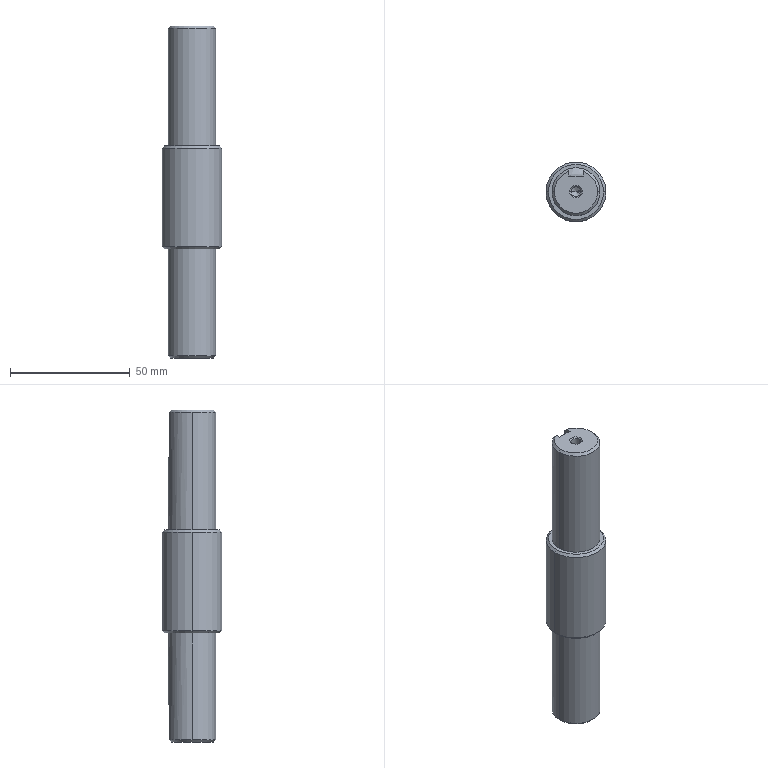Part | SolidWorks | features BaseBody 1 | 1 solid | 40 faces | box 25 x 25 x 138.5 mm | volume 49958 mm3 | cone 18 | cylinder 10 | plane 10 | spline 2 | commonest cylinder face diameters 4.2 x4 20 x4 25 x2
STEP:
#1=CARTESIAN_POINT('',(2.1,0.,-66.5));
#2=VERTEX_POINT('',#1);
#3=CARTESIAN_POINT('',(-2.1,0.,-66.5));
#4=VERTEX_POINT('',#3);
#5=CARTESIAN_POINT('',(0.,0.,-66.5));
#6=DIRECTION('',(0.,0.,-1.));
#7=DIRECTION('',(-1.,0.,0.));
#8=AXIS2_PLACEMENT_3D('',#5,#6,#7);
#9=CIRCLE('',#8,2.1);
#10=EDGE_CURVE('',#2,#4,#9,.T.);
#11=ORIENTED_EDGE('',*,*,#10,.F.);
#12=CARTESIAN_POINT('',(2.6,0.,-67.));
#13=VERTEX_POINT('',#12);
#14=CARTESIAN_POINT('',(2.1,0.,-66.5));
#15=DIRECTION('',(0.7071,0.,-0.7071));
#16=VECTOR('',#15,1000.);
#17=LINE('',#14,#16);
#18=EDGE_CURVE('',#2,#13,#17,.T.);
#19=ORIENTED_EDGE('',*,*,#18,.T.);
#20=CARTESIAN_POINT('',(-2.6,0.,-67.));
#21=VERTEX_POINT('',#20);
#22=CARTESIAN_POINT('',(0.,0.,-67.));
#23=DIRECTION('',(0.,0.,1.));
#24=DIRECTION('',(-1.,0.,0.));
#25=AXIS2_PLACEMENT_3D('',#22,#23,#24);
#26=CIRCLE('',#25,2.6);
#27=EDGE_CURVE('',#21,#13,#26,.T.);
#28=ORIENTED_EDGE('',*,*,#27,.F.);
#29=CARTESIAN_POINT('',(-2.1,0.,-66.5));
#30=DIRECTION('',(-0.7071,0.,-0.7071));
#31=VECTOR('',#30,1000.);
#32=LINE('',#29,#31);
#33=EDGE_CURVE('',#4,#21,#32,.T.);
#34=ORIENTED_EDGE('',*,*,#33,.F.);
#35=EDGE_LOOP('',(#11,#19,#28,#34));
#36=FACE_OUTER_BOUND('',#35,.T.);
#37=CARTESIAN_POINT('',(0.,0.,-66.5));
#38=DIRECTION('',(0.,0.,-1.));
#39=DIRECTION('',(-1.,0.,0.));
#40=AXIS2_PLACEMENT_3D('',#37,#38,#39);
#41=CONICAL_SURFACE('',#40,2.1,0.7854);
#42=ADVANCED_FACE('',(#36),#41,.F.);
#43=CARTESIAN_POINT('',(-2.1,0.,71.));
#44=VERTEX_POINT('',#43);
#45=CARTESIAN_POINT('',(2.1,0.,71.));
#46=VERTEX_POINT('',#45);
#47=CARTESIAN_POINT('',(0.,0.,71.));
#48=DIRECTION('',(0.,0.,1.));
#49=DIRECTION('',(1.,0.,0.));
#50=AXIS2_PLACEMENT_3D('',#47,#48,#49);
#51=CIRCLE('',#50,2.1);
#52=EDGE_CURVE('',#44,#46,#51,.T.);
#53=ORIENTED_EDGE('',*,*,#52,.F.);
#54=CARTESIAN_POINT('',(-2.6,0.,71.5));
#55=VERTEX_POINT('',#54);
#56=CARTESIAN_POINT('',(-2.1,0.,71.));
#57=DIRECTION('',(-0.7071,0.,0.7071));
#58=VECTOR('',#57,1000.);
#59=LINE('',#56,#58);
#60=EDGE_CURVE('',#44,#55,#59,.T.);
#61=ORIENTED_EDGE('',*,*,#60,.T.);
#62=CARTESIAN_POINT('',(2.6,0.,71.5));
#63=VERTEX_POINT('',#62);
#64=CARTESIAN_POINT('',(0.,0.,71.5));
#65=DIRECTION('',(0.,0.,-1.));
#66=DIRECTION('',(1.,0.,0.));
#67=AXIS2_PLACEMENT_3D('',#64,#65,#66);
#68=CIRCLE('',#67,2.6);
#69=EDGE_CURVE('',#63,#55,#68,.T.);
#70=ORIENTED_EDGE('',*,*,#69,.F.);
#71=CARTESIAN_POINT('',(2.1,0.,71.));
#72=DIRECTION('',(0.7071,0.,0.7071));
#73=VECTOR('',#72,1000.);
#74=LINE('',#71,#73);
#75=EDGE_CURVE('',#46,#63,#74,.T.);
#76=ORIENTED_EDGE('',*,*,#75,.F.);
#77=EDGE_LOOP('',(#53,#61,#70,#76));
#78=FACE_OUTER_BOUND('',#77,.T.);
#79=CARTESIAN_POINT('',(0.,0.,71.));
#80=DIRECTION('',(0.,0.,1.));
#81=DIRECTION('',(1.,0.,0.));
#82=AXIS2_PLACEMENT_3D('',#79,#80,#81);
#83=CONICAL_SURFACE('',#82,2.1,0.7854);
#84=ADVANCED_FACE('',(#78),#83,.F.);
#85=CARTESIAN_POINT('',(-2.1,0.,59.1));
#86=VERTEX_POINT('',#85);
#87=CARTESIAN_POINT('',(2.1,0.,59.1));
#88=VERTEX_POINT('',#87);
#89=CARTESIAN_POINT('',(0.,0.,59.1));
#90=DIRECTION('',(0.,0.,1.));
#91=DIRECTION('',(1.,0.,0.));
#92=AXIS2_PLACEMENT_3D('',#89,#90,#91);
#93=CIRCLE('',#92,2.1);
#94=EDGE_CURVE('',#86,#88,#93,.T.);
#95=ORIENTED_EDGE('',*,*,#94,.F.);
#96=CARTESIAN_POINT('',(-2.1,0.,71.5));
#97=DIRECTION('',(0.,0.,1.));
#98=VECTOR('',#97,1000.);
#99=LINE('',#96,#98);
#100=EDGE_CURVE('',#86,#44,#99,.T.);
#101=ORIENTED_EDGE('',*,*,#100,.T.);
#102=ORIENTED_EDGE('',*,*,#52,.T.);
#103=CARTESIAN_POINT('',(2.1,0.,71.5));
#104=DIRECTION('',(0.,0.,1.));
#105=VECTOR('',#104,1000.);
#106=LINE('',#103,#105);
#107=EDGE_CURVE('',#88,#46,#106,.T.);
#108=ORIENTED_EDGE('',*,*,#107,.F.);
#109=EDGE_LOOP('',(#95,#101,#102,#108));
#110=FACE_OUTER_BOUND('',#109,.T.);
#111=CARTESIAN_POINT('',(0.,0.,71.5));
#112=DIRECTION('',(0.,0.,1.));
#113=DIRECTION('',(1.,0.,0.));
#114=AXIS2_PLACEMENT_3D('',#111,#112,#113);
#115=CYLINDRICAL_SURFACE('',#114,2.1);
#116=ADVANCED_FACE('',(#110),#115,.F.);
#117=CARTESIAN_POINT('',(0.,0.,57.838));
#118=VERTEX_POINT('',#117);
#119=CARTESIAN_POINT('',(2.1,0.,59.1));
#120=DIRECTION('',(0.8572,0.,0.515));
#121=VECTOR('',#120,1000.);
#122=LINE('',#119,#121);
#123=EDGE_CURVE('',#118,#88,#122,.T.);
#124=ORIENTED_EDGE('',*,*,#123,.F.);
#125=CARTESIAN_POINT('',(-2.1,0.,59.1));
#126=DIRECTION('',(-0.8572,0.,0.515));
#127=VECTOR('',#126,1000.);
#128=LINE('',#125,#127);
#129=EDGE_CURVE('',#118,#86,#128,.T.);
#130=ORIENTED_EDGE('',*,*,#129,.T.);
#131=ORIENTED_EDGE('',*,*,#94,.T.);
#132=EDGE_LOOP('',(#124,#130,#131));
#133=FACE_OUTER_BOUND('',#132,.T.);
#134=CARTESIAN_POINT('',(0.,0.,59.1));
#135=DIRECTION('',(0.,0.,1.));
#136=DIRECTION('',(1.,0.,0.));
#137=AXIS2_PLACEMENT_3D('',#134,#135,#136);
#138=CONICAL_SURFACE('',#137,2.1,1.03);
#139=ADVANCED_FACE('',(#133),#138,.F.);
#140=CARTESIAN_POINT('',(2.1,0.,-54.6));
#141=VERTEX_POINT('',#140);
#142=CARTESIAN_POINT('',(-2.1,0.,-54.6));
#143=VERTEX_POINT('',#142);
#144=CARTESIAN_POINT('',(0.,0.,-54.6));
#145=DIRECTION('',(0.,0.,-1.));
#146=DIRECTION('',(-1.,0.,0.));
#147=AXIS2_PLACEMENT_3D('',#144,#145,#146);
#148=CIRCLE('',#147,2.1);
#149=EDGE_CURVE('',#141,#143,#148,.T.);
#150=ORIENTED_EDGE('',*,*,#149,.F.);
#151=CARTESIAN_POINT('',(2.1,0.,-67.));
#152=DIRECTION('',(0.,0.,-1.));
#153=VECTOR('',#152,1000.);
#154=LINE('',#151,#153);
#155=EDGE_CURVE('',#141,#2,#154,.T.);
#156=ORIENTED_EDGE('',*,*,#155,.T.);
#157=ORIENTED_EDGE('',*,*,#10,.T.);
#158=CARTESIAN_POINT('',(-2.1,0.,-67.));
#159=DIRECTION('',(0.,0.,-1.));
#160=VECTOR('',#159,1000.);
#161=LINE('',#158,#160);
#162=EDGE_CURVE('',#143,#4,#161,.T.);
#163=ORIENTED_EDGE('',*,*,#162,.F.);
#164=EDGE_LOOP('',(#150,#156,#157,#163));
#165=FACE_OUTER_BOUND('',#164,.T.);
#166=CARTESIAN_POINT('',(0.,0.,-67.));
#167=DIRECTION('',(0.,0.,-1.));
#168=DIRECTION('',(-1.,0.,0.));
#169=AXIS2_PLACEMENT_3D('',#166,#167,#168);
#170=CYLINDRICAL_SURFACE('',#169,2.1);
#171=ADVANCED_FACE('',(#165),#170,.F.);
#172=CARTESIAN_POINT('',(0.,0.,-53.338));
#173=VERTEX_POINT('',#172);
#174=CARTESIAN_POINT('',(-2.1,0.,-54.6));
#175=DIRECTION('',(-0.8572,0.,-0.515));
#176=VECTOR('',#175,1000.);
#177=LINE('',#174,#176);
#178=EDGE_CURVE('',#173,#143,#177,.T.);
#179=ORIENTED_EDGE('',*,*,#178,.F.);
#180=CARTESIAN_POINT('',(2.1,0.,-54.6));
#181=DIRECTION('',(0.8572,0.,-0.515));
#182=VECTOR('',#181,1000.);
#183=LINE('',#180,#182);
#184=EDGE_CURVE('',#173,#141,#183,.T.);
#185=ORIENTED_EDGE('',*,*,#184,.T.);
#186=ORIENTED_EDGE('',*,*,#149,.T.);
#187=EDGE_LOOP('',(#179,#185,#186));
#188=FACE_OUTER_BOUND('',#187,.T.);
#189=CARTESIAN_POINT('',(0.,0.,-54.6));
#190=DIRECTION('',(0.,0.,-1.));
#191=DIRECTION('',(-1.,0.,0.));
#192=AXIS2_PLACEMENT_3D('',#189,#190,#191);
#193=CONICAL_SURFACE('',#192,2.1,1.03);
#194=ADVANCED_FACE('',(#188),#193,.F.);
#195=CARTESIAN_POINT('',(-9.,0.,-67.));
#196=VERTEX_POINT('',#195);
#197=CARTESIAN_POINT('',(-3.,8.485,-67.));
#198=VERTEX_POINT('',#197);
#199=CARTESIAN_POINT('',(0.,0.,-67.));
#200=DIRECTION('',(0.,0.,-1.));
#201=DIRECTION('',(-1.,0.,0.));
#202=AXIS2_PLACEMENT_3D('',#199,#200,#201);
#203=CIRCLE('',#202,9.);
#204=EDGE_CURVE('',#196,#198,#203,.T.);
#205=ORIENTED_EDGE('',*,*,#204,.F.);
#206=CARTESIAN_POINT('',(-10.,0.,-66.));
#207=VERTEX_POINT('',#206);
#208=CARTESIAN_POINT('',(-10.,0.,-66.));
#209=DIRECTION('',(-0.7071,0.,0.7071));
#210=VECTOR('',#209,1000.);
#211=LINE('',#208,#210);
#212=EDGE_CURVE('',#196,#207,#211,.T.);
#213=ORIENTED_EDGE('',*,*,#212,.T.);
#214=CARTESIAN_POINT('',(-3.,9.539,-66.));
#215=VERTEX_POINT('',#214);
#216=CARTESIAN_POINT('',(0.,0.,-66.));
#217=DIRECTION('',(0.,0.,1.));
#218=DIRECTION('',(-1.,0.,0.));
#219=AXIS2_PLACEMENT_3D('',#216,#217,#218);
#220=CIRCLE('',#219,10.);
#221=EDGE_CURVE('',#215,#207,#220,.T.);
#222=ORIENTED_EDGE('',*,*,#221,.F.);
#223=CARTESIAN_POINT('',(-3.,8.485,-67.));
#224=CARTESIAN_POINT('',(-3.,8.838,-66.668));
#225=CARTESIAN_POINT('',(-3.,9.189,-66.334));
#226=CARTESIAN_POINT('',(-3.,9.539,-66.));
#227=B_SPLINE_CURVE_WITH_KNOTS('',3,(#223,#224,#225,#226),.UNSPECIFIED.,.F.,.F.,(4,4),(0.,0.001453),.UNSPECIFIED.);
#228=EDGE_CURVE('',#198,#215,#227,.T.);
#229=ORIENTED_EDGE('',*,*,#228,.F.);
#230=EDGE_LOOP('',(#205,#213,#222,#229));
#231=FACE_OUTER_BOUND('',#230,.T.);
#232=CARTESIAN_POINT('',(0.,0.,-66.));
#233=DIRECTION('',(0.,0.,1.));
#234=DIRECTION('',(1.,0.,0.));
#235=AXIS2_PLACEMENT_3D('',#232,#233,#234);
#236=CONICAL_SURFACE('',#235,10.,0.7854);
#237=ADVANCED_FACE('',(#231),#236,.T.);
#238=ORIENTED_EDGE('',*,*,#212,.F.);
#239=CARTESIAN_POINT('',(9.,0.,-67.));
#240=VERTEX_POINT('',#239);
#241=CARTESIAN_POINT('',(0.,0.,-67.));
#242=DIRECTION('',(0.,0.,-1.));
#243=DIRECTION('',(-1.,0.,0.));
#244=AXIS2_PLACEMENT_3D('',#241,#242,#243);
#245=CIRCLE('',#244,9.);
#246=EDGE_CURVE('',#240,#196,#245,.T.);
#247=ORIENTED_EDGE('',*,*,#246,.F.);
#248=CARTESIAN_POINT('',(10.,0.,-66.));
#249=VERTEX_POINT('',#248);
#250=CARTESIAN_POINT('',(10.,0.,-66.));
#251=DIRECTION('',(0.7071,0.,0.7071));
#252=VECTOR('',#251,1000.);
#253=LINE('',#250,#252);
#254=EDGE_CURVE('',#240,#249,#253,.T.);
#255=ORIENTED_EDGE('',*,*,#254,.T.);
#256=CARTESIAN_POINT('',(0.,0.,-66.));
#257=DIRECTION('',(0.,0.,1.));
#258=DIRECTION('',(-1.,0.,0.));
#259=AXIS2_PLACEMENT_3D('',#256,#257,#258);
#260=CIRCLE('',#259,10.);
#261=EDGE_CURVE('',#207,#249,#260,.T.);
#262=ORIENTED_EDGE('',*,*,#261,.F.);
#263=EDGE_LOOP('',(#238,#247,#255,#262));
#264=FACE_OUTER_BOUND('',#263,.T.);
#265=CARTESIAN_POINT('',(0.,0.,-66.));
#266=DIRECTION('',(0.,0.,1.));
#267=DIRECTION('',(1.,0.,0.));
#268=AXIS2_PLACEMENT_3D('',#265,#266,#267);
#269=CONICAL_SURFACE('',#268,10.,0.7854);
#270=ADVANCED_FACE('',(#264),#269,.T.);
#271=CARTESIAN_POINT('',(11.5,0.,21.5));
#272=VERTEX_POINT('',#271);
#273=CARTESIAN_POINT('',(-11.5,0.,21.5));
#274=VERTEX_POINT('',#273);
#275=CARTESIAN_POINT('',(0.,0.,21.5));
#276=DIRECTION('',(0.,0.,1.));
#277=DIRECTION('',(1.,0.,0.));
#278=AXIS2_PLACEMENT_3D('',#275,#276,#277);
#279=CIRCLE('',#278,11.5);
#280=EDGE_CURVE('',#272,#274,#279,.T.);
#281=ORIENTED_EDGE('',*,*,#280,.F.);
#282=CARTESIAN_POINT('',(12.5,0.,20.5));
#283=VERTEX_POINT('',#282);
#284=CARTESIAN_POINT('',(11.5,0.,21.5));
#285=DIRECTION('',(0.7071,0.,-0.7071));
#286=VECTOR('',#285,1000.);
#287=LINE('',#284,#286);
#288=EDGE_CURVE('',#272,#283,#287,.T.);
#289=ORIENTED_EDGE('',*,*,#288,.T.);
#290=CARTESIAN_POINT('',(-12.5,0.,20.5));
#291=VERTEX_POINT('',#290);
#292=CARTESIAN_POINT('',(0.,0.,20.5));
#293=DIRECTION('',(0.,0.,-1.));
#294=DIRECTION('',(1.,0.,0.));
#295=AXIS2_PLACEMENT_3D('',#292,#293,#294);
#296=CIRCLE('',#295,12.5);
#297=EDGE_CURVE('',#291,#283,#296,.T.);
#298=ORIENTED_EDGE('',*,*,#297,.F.);
#299=CARTESIAN_POINT('',(-11.5,0.,21.5));
#300=DIRECTION('',(-0.7071,0.,-0.7071));
#301=VECTOR('',#300,1000.);
#302=LINE('',#299,#301);
#303=EDGE_CURVE('',#274,#291,#302,.T.);
#304=ORIENTED_EDGE('',*,*,#303,.F.);
#305=EDGE_LOOP('',(#281,#289,#298,#304));
#306=FACE_OUTER_BOUND('',#305,.T.);
#307=CARTESIAN_POINT('',(0.,0.,21.5));
#308=DIRECTION('',(0.,0.,-1.));
#309=DIRECTION('',(-1.,0.,0.));
#310=AXIS2_PLACEMENT_3D('',#307,#308,#309);
#311=CONICAL_SURFACE('',#310,11.5,0.7854);
#312=ADVANCED_FACE('',(#306),#311,.T.);
#313=CARTESIAN_POINT('',(-11.5,0.,-21.5));
#314=VERTEX_POINT('',#313);
#315=CARTESIAN_POINT('',(11.5,0.,-21.5));
#316=VERTEX_POINT('',#315);
#317=CARTESIAN_POINT('',(0.,0.,-21.5));
#318=DIRECTION('',(0.,0.,-1.));
#319=DIRECTION('',(1.,0.,0.));
#320=AXIS2_PLACEMENT_3D('',#317,#318,#319);
#321=CIRCLE('',#320,11.5);
#322=EDGE_CURVE('',#314,#316,#321,.T.);
#323=ORIENTED_EDGE('',*,*,#322,.F.);
#324=CARTESIAN_POINT('',(-12.5,0.,-20.5));
#325=VERTEX_POINT('',#324);
#326=CARTESIAN_POINT('',(-12.5,0.,-20.5));
#327=DIRECTION('',(-0.7071,0.,0.7071));
#328=VECTOR('',#327,1000.);
#329=LINE('',#326,#328);
#330=EDGE_CURVE('',#314,#325,#329,.T.);
#331=ORIENTED_EDGE('',*,*,#330,.T.);
#332=CARTESIAN_POINT('',(12.5,0.,-20.5));
#333=VERTEX_POINT('',#332);
#334=CARTESIAN_POINT('',(0.,0.,-20.5));
#335=DIRECTION('',(0.,0.,1.));
#336=DIRECTION('',(1.,0.,0.));
#337=AXIS2_PLACEMENT_3D('',#334,#335,#336);
#338=CIRCLE('',#337,12.5);
#339=EDGE_CURVE('',#333,#325,#338,.T.);
#340=ORIENTED_EDGE('',*,*,#339,.F.);
#341=CARTESIAN_POINT('',(12.5,0.,-20.5));
#342=DIRECTION('',(0.7071,0.,0.7071));
#343=VECTOR('',#342,1000.);
#344=LINE('',#341,#343);
#345=EDGE_CURVE('',#316,#333,#344,.T.);
#346=ORIENTED_EDGE('',*,*,#345,.F.);
#347=EDGE_LOOP('',(#323,#331,#340,#346));
#348=FACE_OUTER_BOUND('',#347,.T.);
#349=CARTESIAN_POINT('',(0.,0.,-20.5));
#350=DIRECTION('',(0.,0.,1.));
#351=DIRECTION('',(1.,0.,0.));
#352=AXIS2_PLACEMENT_3D('',#349,#350,#351);
#353=CONICAL_SURFACE('',#352,12.5,0.7854);
#354=ADVANCED_FACE('',(#348),#353,.T.);
#355=CARTESIAN_POINT('',(9.,0.,71.5));
#356=VERTEX_POINT('',#355);
#357=CARTESIAN_POINT('',(3.,8.485,71.5));
#358=VERTEX_POINT('',#357);
#359=CARTESIAN_POINT('',(0.,0.,71.5));
#360=DIRECTION('',(0.,0.,1.));
#361=DIRECTION('',(1.,0.,0.));
#362=AXIS2_PLACEMENT_3D('',#359,#360,#361);
#363=CIRCLE('',#362,9.);
#364=EDGE_CURVE('',#356,#358,#363,.T.);
#365=ORIENTED_EDGE('',*,*,#364,.F.);
#366=CARTESIAN_POINT('',(10.,0.,70.5));
#367=VERTEX_POINT('',#366);
#368=CARTESIAN_POINT('',(9.,0.,71.5));
#369=DIRECTION('',(0.7071,0.,-0.7071));
#370=VECTOR('',#369,1000.);
#371=LINE('',#368,#370);
#372=EDGE_CURVE('',#356,#367,#371,.T.);
#373=ORIENTED_EDGE('',*,*,#372,.T.);
#374=CARTESIAN_POINT('',(3.,9.539,70.5));
#375=VERTEX_POINT('',#374);
#376=CARTESIAN_POINT('',(0.,0.,70.5));
#377=DIRECTION('',(0.,0.,-1.));
#378=DIRECTION('',(1.,0.,0.));
#379=AXIS2_PLACEMENT_3D('',#376,#377,#378);
#380=CIRCLE('',#379,10.);
#381=EDGE_CURVE('',#375,#367,#380,.T.);
#382=ORIENTED_EDGE('',*,*,#381,.F.);
#383=CARTESIAN_POINT('',(3.,8.485,71.5));
#384=CARTESIAN_POINT('',(3.,8.838,71.168));
#385=CARTESIAN_POINT('',(3.,9.189,70.834));
#386=CARTESIAN_POINT('',(3.,9.539,70.5));
#387=B_SPLINE_CURVE_WITH_KNOTS('',3,(#383,#384,#385,#386),.UNSPECIFIED.,.F.,.F.,(4,4),(0.006491,0.007944),.UNSPECIFIED.);
#388=EDGE_CURVE('',#358,#375,#387,.T.);
#389=ORIENTED_EDGE('',*,*,#388,.F.);
#390=EDGE_LOOP('',(#365,#373,#382,#389));
#391=FACE_OUTER_BOUND('',#390,.T.);
#392=CARTESIAN_POINT('',(0.,0.,71.5));
#393=DIRECTION('',(0.,0.,-1.));
#394=DIRECTION('',(-1.,0.,0.));
#395=AXIS2_PLACEMENT_3D('',#392,#393,#394);
#396=CONICAL_SURFACE('',#395,9.,0.7854);
#397=ADVANCED_FACE('',(#391),#396,.T.);
#398=ORIENTED_EDGE('',*,*,#372,.F.);
#399=CARTESIAN_POINT('',(-9.,0.,71.5));
#400=VERTEX_POINT('',#399);
#401=CARTESIAN_POINT('',(0.,0.,71.5));
#402=DIRECTION('',(0.,0.,1.));
#403=DIRECTION('',(1.,0.,0.));
#404=AXIS2_PLACEMENT_3D('',#401,#402,#403);
#405=CIRCLE('',#404,9.);
#406=EDGE_CURVE('',#400,#356,#405,.T.);
#407=ORIENTED_EDGE('',*,*,#406,.F.);
#408=CARTESIAN_POINT('',(-10.,0.,70.5));
#409=VERTEX_POINT('',#408);
#410=CARTESIAN_POINT('',(-9.,0.,71.5));
#411=DIRECTION('',(-0.7071,0.,-0.7071));
#412=VECTOR('',#411,1000.);
#413=LINE('',#410,#412);
#414=EDGE_CURVE('',#400,#409,#413,.T.);
#415=ORIENTED_EDGE('',*,*,#414,.T.);
#416=CARTESIAN_POINT('',(0.,0.,70.5));
#417=DIRECTION('',(0.,0.,-1.));
#418=DIRECTION('',(1.,0.,0.));
#419=AXIS2_PLACEMENT_3D('',#416,#417,#418);
#420=CIRCLE('',#419,10.);
#421=EDGE_CURVE('',#367,#409,#420,.T.);
#422=ORIENTED_EDGE('',*,*,#421,.F.);
#423=EDGE_LOOP('',(#398,#407,#415,#422));
#424=FACE_OUTER_BOUND('',#423,.T.);
#425=CARTESIAN_POINT('',(0.,0.,71.5));
#426=DIRECTION('',(0.,0.,-1.));
#427=DIRECTION('',(-1.,0.,0.));
#428=AXIS2_PLACEMENT_3D('',#425,#426,#427);
#429=CONICAL_SURFACE('',#428,9.,0.7854);
#430=ADVANCED_FACE('',(#424),#429,.T.);
#431=ORIENTED_EDGE('',*,*,#381,.T.);
#432=CARTESIAN_POINT('',(10.,0.,21.5));
#433=VERTEX_POINT('',#432);
#434=CARTESIAN_POINT('',(10.,0.,71.5));
#435=DIRECTION('',(0.,0.,-1.));
#436=VECTOR('',#435,1000.);
#437=LINE('',#434,#436);
#438=EDGE_CURVE('',#367,#433,#437,.T.);
#439=ORIENTED_EDGE('',*,*,#438,.T.);
#440=CARTESIAN_POINT('',(-10.,0.,21.5));
#441=VERTEX_POINT('',#440);
#442=CARTESIAN_POINT('',(0.,0.,21.5));
#443=DIRECTION('',(0.,0.,1.));
#444=DIRECTION('',(1.,0.,0.));
#445=AXIS2_PLACEMENT_3D('',#442,#443,#444);
#446=CIRCLE('',#445,10.);
#447=EDGE_CURVE('',#433,#441,#446,.T.);
#448=ORIENTED_EDGE('',*,*,#447,.T.);
#449=CARTESIAN_POINT('',(-10.,0.,71.5));
#450=DIRECTION('',(0.,0.,-1.));
#451=VECTOR('',#450,1000.);
#452=LINE('',#449,#451);
#453=EDGE_CURVE('',#409,#441,#452,.T.);
#454=ORIENTED_EDGE('',*,*,#453,.F.);
#455=CARTESIAN_POINT('',(-3.,9.539,70.5));
#456=VERTEX_POINT('',#455);
#457=CARTESIAN_POINT('',(0.,0.,70.5));
#458=DIRECTION('',(0.,0.,-1.));
#459=DIRECTION('',(1.,0.,0.));
#460=AXIS2_PLACEMENT_3D('',#457,#458,#459);
#461=CIRCLE('',#460,10.);
#462=EDGE_CURVE('',#409,#456,#461,.T.);
#463=ORIENTED_EDGE('',*,*,#462,.T.);
#464=CARTESIAN_POINT('',(-3.,9.539,51.5));
#465=VERTEX_POINT('',#464);
#466=CARTESIAN_POINT('',(-3.,9.539,71.5));
#467=DIRECTION('',(0.,0.,-1.));
#468=VECTOR('',#467,1000.);
#469=LINE('',#466,#468);
#470=EDGE_CURVE('',#456,#465,#469,.T.);
#471=ORIENTED_EDGE('',*,*,#470,.T.);
#472=CARTESIAN_POINT('',(3.,9.539,51.5));
#473=VERTEX_POINT('',#472);
#474=CARTESIAN_POINT('',(-3.,9.539,51.5));
#475=CARTESIAN_POINT('',(-2.514,9.692,51.5));
#476=CARTESIAN_POINT('',(-2.019,9.807,51.5));
#477=CARTESIAN_POINT('',(-1.011,9.962,51.5));
#478=CARTESIAN_POINT('',(-0.5036,10.,51.5));
#479=CARTESIAN_POINT('',(0.5143,10.,51.5));
#480=CARTESIAN_POINT('',(1.022,9.96,51.5));
#481=CARTESIAN_POINT('',(2.021,9.807,51.5));
#482=CARTESIAN_POINT('',(2.514,9.692,51.5));
#483=CARTESIAN_POINT('',(3.,9.539,51.5));
#484=B_SPLINE_CURVE_WITH_KNOTS('',3,(#474,#475,#476,#477,#478,#479,#480,#481,#482,#483),.UNSPECIFIED.,.F.,.F.,(4,2,2,2,4),(0.,0.001525,0.003049,0.004574,0.006098),.UNSPECIFIED.);
#485=EDGE_CURVE('',#465,#473,#484,.T.);
#486=ORIENTED_EDGE('',*,*,#485,.T.);
#487=CARTESIAN_POINT('',(3.,9.539,71.5));
#488=DIRECTION('',(0.,0.,1.));
#489=VECTOR('',#488,1000.);
#490=LINE('',#487,#489);
#491=EDGE_CURVE('',#473,#375,#490,.T.);
#492=ORIENTED_EDGE('',*,*,#491,.T.);
#493=EDGE_LOOP('',(#431,#439,#448,#454,#463,#471,#486,#492));
#494=FACE_OUTER_BOUND('',#493,.T.);
#495=CARTESIAN_POINT('',(0.,0.,71.5));
#496=DIRECTION('',(0.,0.,-1.));
#497=DIRECTION('',(-1.,0.,0.));
#498=AXIS2_PLACEMENT_3D('',#495,#496,#497);
#499=CYLINDRICAL_SURFACE('',#498,10.);
#500=ADVANCED_FACE('',(#494),#499,.T.);
#501=ORIENTED_EDGE('',*,*,#297,.T.);
#502=CARTESIAN_POINT('',(12.5,0.,21.5));
#503=DIRECTION('',(0.,0.,-1.));
#504=VECTOR('',#503,1000.);
#505=LINE('',#502,#504);
#506=EDGE_CURVE('',#283,#333,#505,.T.);
#507=ORIENTED_EDGE('',*,*,#506,.T.);
#508=ORIENTED_EDGE('',*,*,#339,.T.);
#509=CARTESIAN_POINT('',(-12.5,0.,21.5));
#510=DIRECTION('',(0.,0.,-1.));
#511=VECTOR('',#510,1000.);
#512=LINE('',#509,#511);
#513=EDGE_CURVE('',#291,#325,#512,.T.);
#514=ORIENTED_EDGE('',*,*,#513,.F.);
#515=EDGE_LOOP('',(#501,#507,#508,#514));
#516=FACE_OUTER_BOUND('',#515,.T.);
#517=CARTESIAN_POINT('',(0.,0.,21.5));
#518=DIRECTION('',(0.,0.,-1.));
#519=DIRECTION('',(-1.,0.,0.));
#520=AXIS2_PLACEMENT_3D('',#517,#518,#519);
#521=CYLINDRICAL_SURFACE('',#520,12.5);
#522=ADVANCED_FACE('',(#516),#521,.T.);
#523=ORIENTED_EDGE('',*,*,#221,.T.);
#524=CARTESIAN_POINT('',(-10.,0.,-21.5));
#525=VERTEX_POINT('',#524);
#526=CARTESIAN_POINT('',(-10.,0.,-71.5));
#527=DIRECTION('',(0.,0.,1.));
#528=VECTOR('',#527,1000.);
#529=LINE('',#526,#528);
#530=EDGE_CURVE('',#207,#525,#529,.T.);
#531=ORIENTED_EDGE('',*,*,#530,.T.);
#532=CARTESIAN_POINT('',(10.,0.,-21.5));
#533=VERTEX_POINT('',#532);
#534=CARTESIAN_POINT('',(0.,0.,-21.5));
#535=DIRECTION('',(0.,0.,1.));
#536=DIRECTION('',(1.,0.,0.));
#537=AXIS2_PLACEMENT_3D('',#534,#535,#536);
#538=CIRCLE('',#537,10.);
#539=EDGE_CURVE('',#533,#525,#538,.T.);
#540=ORIENTED_EDGE('',*,*,#539,.F.);
#541=CARTESIAN_POINT('',(10.,0.,-71.5));
#542=DIRECTION('',(0.,0.,1.));
#543=VECTOR('',#542,1000.);
#544=LINE('',#541,#543);
#545=EDGE_CURVE('',#249,#533,#544,.T.);
#546=ORIENTED_EDGE('',*,*,#545,.F.);
#547=CARTESIAN_POINT('',(3.,9.539,-66.));
#548=VERTEX_POINT('',#547);
#549=CARTESIAN_POINT('',(0.,0.,-66.));
#550=DIRECTION('',(0.,0.,1.));
#551=DIRECTION('',(-1.,0.,0.));
#552=AXIS2_PLACEMENT_3D('',#549,#550,#551);
#553=CIRCLE('',#552,10.);
#554=EDGE_CURVE('',#249,#548,#553,.T.);
#555=ORIENTED_EDGE('',*,*,#554,.T.);
#556=CARTESIAN_POINT('',(3.,9.539,-51.5));
#557=VERTEX_POINT('',#556);
#558=CARTESIAN_POINT('',(3.,9.539,-71.5));
#559=DIRECTION('',(0.,0.,1.));
#560=VECTOR('',#559,1000.);
#561=LINE('',#558,#560);
#562=EDGE_CURVE('',#548,#557,#561,.T.);
#563=ORIENTED_EDGE('',*,*,#562,.T.);
#564=CARTESIAN_POINT('',(-3.,9.539,-51.5));
#565=VERTEX_POINT('',#564);
#566=CARTESIAN_POINT('',(-3.,9.539,-51.5));
#567=CARTESIAN_POINT('',(-2.514,9.692,-51.5));
#568=CARTESIAN_POINT('',(-2.019,9.807,-51.5));
#569=CARTESIAN_POINT('',(-1.011,9.962,-51.5));
#570=CARTESIAN_POINT('',(-0.5036,10.,-51.5));
#571=CARTESIAN_POINT('',(0.5143,10.,-51.5));
#572=CARTESIAN_POINT('',(1.022,9.96,-51.5));
#573=CARTESIAN_POINT('',(2.021,9.807,-51.5));
#574=CARTESIAN_POINT('',(2.514,9.692,-51.5));
#575=CARTESIAN_POINT('',(3.,9.539,-51.5));
#576=B_SPLINE_CURVE_WITH_KNOTS('',3,(#566,#567,#568,#569,#570,#571,#572,#573,#574,#575),.UNSPECIFIED.,.F.,.F.,(4,2,2,2,4),(0.,0.001525,0.003049,0.004574,0.006098),.UNSPECIFIED.);
#577=EDGE_CURVE('',#565,#557,#576,.T.);
#578=ORIENTED_EDGE('',*,*,#577,.F.);
#579=CARTESIAN_POINT('',(-3.,9.539,-71.5));
#580=DIRECTION('',(0.,0.,-1.));
#581=VECTOR('',#580,1000.);
#582=LINE('',#579,#581);
#583=EDGE_CURVE('',#565,#215,#582,.T.);
#584=ORIENTED_EDGE('',*,*,#583,.T.);
#585=EDGE_LOOP('',(#523,#531,#540,#546,#555,#563,#578,#584));
#586=FACE_OUTER_BOUND('',#585,.T.);
#587=CARTESIAN_POINT('',(0.,0.,-71.5));
#588=DIRECTION('',(0.,0.,1.));
#589=DIRECTION('',(1.,0.,0.));
#590=AXIS2_PLACEMENT_3D('',#587,#588,#589);
#591=CYLINDRICAL_SURFACE('',#590,10.);
#592=ADVANCED_FACE('',(#586),#591,.T.);
#593=ORIENTED_EDGE('',*,*,#27,.T.);
#594=CARTESIAN_POINT('',(0.,0.,-67.));
#595=DIRECTION('',(0.,0.,1.));
#596=DIRECTION('',(-1.,0.,0.));
#597=AXIS2_PLACEMENT_3D('',#594,#595,#596);
#598=CIRCLE('',#597,2.6);
#599=EDGE_CURVE('',#13,#21,#598,.T.);
#600=ORIENTED_EDGE('',*,*,#599,.T.);
#601=EDGE_LOOP('',(#593,#600));
#602=FACE_BOUND('',#601,.T.);
#603=CARTESIAN_POINT('',(3.,8.485,-67.));
#604=VERTEX_POINT('',#603);
#605=CARTESIAN_POINT('',(3.,6.5,-67.));
#606=VERTEX_POINT('',#605);
#607=CARTESIAN_POINT('',(3.,6.5,-67.));
#608=DIRECTION('',(0.,-1.,0.));
#609=VECTOR('',#608,1000.);
#610=LINE('',#607,#609);
#611=EDGE_CURVE('',#604,#606,#610,.T.);
#612=ORIENTED_EDGE('',*,*,#611,.F.);
#613=CARTESIAN_POINT('',(0.,0.,-67.));
#614=DIRECTION('',(0.,0.,-1.));
#615=DIRECTION('',(-1.,0.,0.));
#616=AXIS2_PLACEMENT_3D('',#613,#614,#615);
#617=CIRCLE('',#616,9.);
#618=EDGE_CURVE('',#604,#240,#617,.T.);
#619=ORIENTED_EDGE('',*,*,#618,.T.);
#620=ORIENTED_EDGE('',*,*,#246,.T.);
#621=ORIENTED_EDGE('',*,*,#204,.T.);
#622=CARTESIAN_POINT('',(-3.,6.5,-67.));
#623=VERTEX_POINT('',#622);
#624=CARTESIAN_POINT('',(-3.,6.5,-67.));
#625=DIRECTION('',(0.,1.,0.));
#626=VECTOR('',#625,1000.);
#627=LINE('',#624,#626);
#628=EDGE_CURVE('',#623,#198,#627,.T.);
#629=ORIENTED_EDGE('',*,*,#628,.F.);
#630=CARTESIAN_POINT('',(-3.,6.5,-67.));
#631=DIRECTION('',(-1.,0.,0.));
#632=VECTOR('',#631,1000.);
#633=LINE('',#630,#632);
#634=EDGE_CURVE('',#606,#623,#633,.T.);
#635=ORIENTED_EDGE('',*,*,#634,.F.);
#636=EDGE_LOOP('',(#612,#619,#620,#621,#629,#635));
#637=FACE_OUTER_BOUND('',#636,.T.);
#638=CARTESIAN_POINT('',(0.,0.,-67.));
#639=DIRECTION('',(0.,0.,-1.));
#640=DIRECTION('',(0.,-1.,0.));
#641=AXIS2_PLACEMENT_3D('',#638,#639,#640);
#642=PLANE('',#641);
#643=ADVANCED_FACE('',(#602,#637),#642,.T.);
#644=CARTESIAN_POINT('',(-3.,6.5,56.131));
#645=VERTEX_POINT('',#644);
#646=CARTESIAN_POINT('',(-3.,6.5,56.131));
#647=CARTESIAN_POINT('',(-3.,6.5,55.638));
#648=CARTESIAN_POINT('',(-3.,6.571,55.157));
#649=CARTESIAN_POINT('',(-3.,6.78,54.454));
#650=CARTESIAN_POINT('',(-3.,6.868,54.222));
#651=CARTESIAN_POINT('',(-3.,7.073,53.78));
#652=CARTESIAN_POINT('',(-3.,7.191,53.568));
#653=CARTESIAN_POINT('',(-3.,7.458,53.16));
#654=CARTESIAN_POINT('',(-3.,7.608,52.963));
#655=CARTESIAN_POINT('',(-3.,7.933,52.597));
#656=CARTESIAN_POINT('',(-3.,8.107,52.427));
#657=CARTESIAN_POINT('',(-3.,8.664,51.957));
#658=CARTESIAN_POINT('',(-3.,9.087,51.695));
#659=CARTESIAN_POINT('',(-3.,9.539,51.5));
#660=B_SPLINE_CURVE_WITH_KNOTS('',3,(#646,#647,#648,#649,#650,#651,#652,#653,#654,#655,#656,#657,#658,#659),.UNSPECIFIED.,.F.,.F.,(4,2,2,2,2,2,4),(0.,0.001458,0.002187,0.002916,0.003645,0.004373,0.005831),.UNSPECIFIED.);
#661=EDGE_CURVE('',#645,#465,#660,.T.);
#662=ORIENTED_EDGE('',*,*,#661,.F.);
#663=CARTESIAN_POINT('',(3.,6.5,56.131));
#664=VERTEX_POINT('',#663);
#665=CARTESIAN_POINT('',(3.,6.5,56.131));
#666=CARTESIAN_POINT('',(2.002,6.5,56.234));
#667=CARTESIAN_POINT('',(0.9991,6.5,56.27));
#668=CARTESIAN_POINT('',(-1.002,6.5,56.27));
#669=CARTESIAN_POINT('',(-2.002,6.5,56.234));
#670=CARTESIAN_POINT('',(-3.,6.5,56.131));
#671=B_SPLINE_CURVE_WITH_KNOTS('',3,(#665,#666,#667,#668,#669,#670),.UNSPECIFIED.,.F.,.F.,(4,2,4),(0.,0.003008,0.006016),.UNSPECIFIED.);
#672=EDGE_CURVE('',#664,#645,#671,.T.);
#673=ORIENTED_EDGE('',*,*,#672,.F.);
#674=CARTESIAN_POINT('',(3.,9.539,51.5));
#675=CARTESIAN_POINT('',(3.,9.087,51.695));
#676=CARTESIAN_POINT('',(3.,8.673,51.951));
#677=CARTESIAN_POINT('',(3.,8.111,52.423));
#678=CARTESIAN_POINT('',(3.,7.934,52.596));
#679=CARTESIAN_POINT('',(3.,7.611,52.96));
#680=CARTESIAN_POINT('',(3.,7.463,53.153));
#681=CARTESIAN_POINT('',(3.,7.195,53.561));
#682=CARTESIAN_POINT('',(3.,7.075,53.777));
#683=CARTESIAN_POINT('',(3.,6.869,54.22));
#684=CARTESIAN_POINT('',(3.,6.782,54.448));
#685=CARTESIAN_POINT('',(3.,6.573,55.146));
#686=CARTESIAN_POINT('',(3.,6.5,55.638));
#687=CARTESIAN_POINT('',(3.,6.5,56.131));
#688=B_SPLINE_CURVE_WITH_KNOTS('',3,(#674,#675,#676,#677,#678,#679,#680,#681,#682,#683,#684,#685,#686,#687),.UNSPECIFIED.,.F.,.F.,(4,2,2,2,2,2,4),(0.,0.001458,0.002187,0.002915,0.003644,0.004373,0.005831),.UNSPECIFIED.);
#689=EDGE_CURVE('',#473,#664,#688,.T.);
#690=ORIENTED_EDGE('',*,*,#689,.F.);
#691=ORIENTED_EDGE('',*,*,#485,.F.);
#692=EDGE_LOOP('',(#662,#673,#690,#691));
#693=FACE_OUTER_BOUND('',#692,.T.);
#694=CARTESIAN_POINT('',(-3.032,9.529,51.5));
#695=CARTESIAN_POINT('',(-3.21,6.5,52.787));
#696=CARTESIAN_POINT('',(-3.66,6.5,56.052));
#697=CARTESIAN_POINT('',(-2.577,9.674,51.5));
#698=CARTESIAN_POINT('',(-2.697,6.5,52.742));
#699=CARTESIAN_POINT('',(-3.054,6.5,56.136));
#700=CARTESIAN_POINT('',(-2.088,9.793,51.5));
#701=CARTESIAN_POINT('',(-2.175,6.5,52.694));
#702=CARTESIAN_POINT('',(-2.447,6.5,56.188));
#703=CARTESIAN_POINT('',(-1.069,9.956,51.5));
#704=CARTESIAN_POINT('',(-1.102,6.5,52.622));
#705=CARTESIAN_POINT('',(-1.229,6.5,56.255));
#706=CARTESIAN_POINT('',(-0.5385,10.,51.5));
#707=CARTESIAN_POINT('',(-0.5571,6.5,52.601));
#708=CARTESIAN_POINT('',(-0.6192,6.5,56.27));
#709=CARTESIAN_POINT('',(0.5242,10.,51.5));
#710=CARTESIAN_POINT('',(0.5423,6.5,52.601));
#711=CARTESIAN_POINT('',(0.6028,6.5,56.27));
#712=CARTESIAN_POINT('',(1.056,9.958,51.5));
#713=CARTESIAN_POINT('',(1.089,6.5,52.622));
#714=CARTESIAN_POINT('',(1.215,6.5,56.255));
#715=CARTESIAN_POINT('',(2.084,9.794,51.5));
#716=CARTESIAN_POINT('',(2.17,6.5,52.693));
#717=CARTESIAN_POINT('',(2.441,6.5,56.188));
#718=CARTESIAN_POINT('',(2.576,9.674,51.5));
#719=CARTESIAN_POINT('',(2.696,6.5,52.742));
#720=CARTESIAN_POINT('',(3.052,6.5,56.136));
#721=CARTESIAN_POINT('',(3.033,9.529,51.5));
#722=CARTESIAN_POINT('',(3.21,6.5,52.787));
#723=CARTESIAN_POINT('',(3.66,6.5,56.052));
#724=(BOUNDED_SURFACE()B_SPLINE_SURFACE(3,2,((#694,#695,#696),(#697,#698,#699),(#700,#701,#702),(#703,#704,#705),(#706,#707,#708),(#709,#710,#711),(#712,#713,#714),(#715,#716,#717),(#718,#719,#720),(#721,#722,#723)),.UNSPECIFIED.,.F.,.F.,.T.)B_SPLINE_SURFACE_WITH_KNOTS((4,2,2,2,4),(3,3),(0.008171,0.01002,0.01187,0.01371,0.01556),(0.,1.),.UNSPECIFIED.)GEOMETRIC_REPRESENTATION_ITEM()RATIONAL_B_SPLINE_SURFACE(((1.,0.8349,1.),(1.,0.8262,1.),(1.,0.819,1.),(1.,0.809,1.),(1.,0.8062,1.),(1.,0.8062,1.),(1.,0.8089,1.),(1.,0.8189,1.),(1.,0.8262,1.),(1.,0.8349,1.)))REPRESENTATION_ITEM('')SURFACE());
#725=ADVANCED_FACE('',(#693),#724,.F.);
#726=CARTESIAN_POINT('',(-3.,6.5,-56.131));
#727=VERTEX_POINT('',#726);
#728=CARTESIAN_POINT('',(-3.,9.539,-51.5));
#729=CARTESIAN_POINT('',(-3.,9.087,-51.695));
#730=CARTESIAN_POINT('',(-3.,8.673,-51.951));
#731=CARTESIAN_POINT('',(-3.,8.111,-52.423));
#732=CARTESIAN_POINT('',(-3.,7.934,-52.596));
#733=CARTESIAN_POINT('',(-3.,7.611,-52.96));
#734=CARTESIAN_POINT('',(-3.,7.463,-53.153));
#735=CARTESIAN_POINT('',(-3.,7.195,-53.561));
#736=CARTESIAN_POINT('',(-3.,7.075,-53.777));
#737=CARTESIAN_POINT('',(-3.,6.869,-54.22));
#738=CARTESIAN_POINT('',(-3.,6.782,-54.448));
#739=CARTESIAN_POINT('',(-3.,6.573,-55.146));
#740=CARTESIAN_POINT('',(-3.,6.5,-55.638));
#741=CARTESIAN_POINT('',(-3.,6.5,-56.131));
#742=B_SPLINE_CURVE_WITH_KNOTS('',3,(#728,#729,#730,#731,#732,#733,#734,#735,#736,#737,#738,#739,#740,#741),.UNSPECIFIED.,.F.,.F.,(4,2,2,2,2,2,4),(0.,0.001458,0.002187,0.002915,0.003644,0.004373,0.005831),.UNSPECIFIED.);
#743=EDGE_CURVE('',#565,#727,#742,.T.);
#744=ORIENTED_EDGE('',*,*,#743,.F.);
#745=ORIENTED_EDGE('',*,*,#577,.T.);
#746=CARTESIAN_POINT('',(3.,6.5,-56.131));
#747=VERTEX_POINT('',#746);
#748=CARTESIAN_POINT('',(3.,6.5,-56.131));
#749=CARTESIAN_POINT('',(3.,6.5,-55.638));
#750=CARTESIAN_POINT('',(3.,6.571,-55.157));
#751=CARTESIAN_POINT('',(3.,6.78,-54.454));
#752=CARTESIAN_POINT('',(3.,6.868,-54.222));
#753=CARTESIAN_POINT('',(3.,7.073,-53.78));
#754=CARTESIAN_POINT('',(3.,7.191,-53.568));
#755=CARTESIAN_POINT('',(3.,7.458,-53.16));
#756=CARTESIAN_POINT('',(3.,7.608,-52.963));
#757=CARTESIAN_POINT('',(3.,7.933,-52.597));
#758=CARTESIAN_POINT('',(3.,8.107,-52.427));
#759=CARTESIAN_POINT('',(3.,8.664,-51.957));
#760=CARTESIAN_POINT('',(3.,9.087,-51.695));
#761=CARTESIAN_POINT('',(3.,9.539,-51.5));
#762=B_SPLINE_CURVE_WITH_KNOTS('',3,(#748,#749,#750,#751,#752,#753,#754,#755,#756,#757,#758,#759,#760,#761),.UNSPECIFIED.,.F.,.F.,(4,2,2,2,2,2,4),(0.,0.001458,0.002187,0.002916,0.003645,0.004373,0.005831),.UNSPECIFIED.);
#763=EDGE_CURVE('',#747,#557,#762,.T.);
#764=ORIENTED_EDGE('',*,*,#763,.F.);
#765=CARTESIAN_POINT('',(-3.,6.5,-56.131));
#766=CARTESIAN_POINT('',(-2.002,6.5,-56.234));
#767=CARTESIAN_POINT('',(-0.9991,6.5,-56.27));
#768=CARTESIAN_POINT('',(1.002,6.5,-56.27));
#769=CARTESIAN_POINT('',(2.002,6.5,-56.234));
#770=CARTESIAN_POINT('',(3.,6.5,-56.131));
#771=B_SPLINE_CURVE_WITH_KNOTS('',3,(#765,#766,#767,#768,#769,#770),.UNSPECIFIED.,.F.,.F.,(4,2,4),(0.,0.003008,0.006016),.UNSPECIFIED.);
#772=EDGE_CURVE('',#727,#747,#771,.T.);
#773=ORIENTED_EDGE('',*,*,#772,.F.);
#774=EDGE_LOOP('',(#744,#745,#764,#773));
#775=FACE_OUTER_BOUND('',#774,.T.);
#776=CARTESIAN_POINT('',(3.032,9.529,-51.5));
#777=CARTESIAN_POINT('',(3.21,6.5,-52.787));
#778=CARTESIAN_POINT('',(3.66,6.5,-56.052));
#779=CARTESIAN_POINT('',(2.577,9.674,-51.5));
#780=CARTESIAN_POINT('',(2.697,6.5,-52.742));
#781=CARTESIAN_POINT('',(3.054,6.5,-56.136));
#782=CARTESIAN_POINT('',(2.088,9.793,-51.5));
#783=CARTESIAN_POINT('',(2.175,6.5,-52.694));
#784=CARTESIAN_POINT('',(2.447,6.5,-56.188));
#785=CARTESIAN_POINT('',(1.069,9.956,-51.5));
#786=CARTESIAN_POINT('',(1.102,6.5,-52.622));
#787=CARTESIAN_POINT('',(1.229,6.5,-56.255));
#788=CARTESIAN_POINT('',(0.5385,10.,-51.5));
#789=CARTESIAN_POINT('',(0.5571,6.5,-52.601));
#790=CARTESIAN_POINT('',(0.6192,6.5,-56.27));
#791=CARTESIAN_POINT('',(-0.5242,10.,-51.5));
#792=CARTESIAN_POINT('',(-0.5423,6.5,-52.601));
#793=CARTESIAN_POINT('',(-0.6028,6.5,-56.27));
#794=CARTESIAN_POINT('',(-1.056,9.958,-51.5));
#795=CARTESIAN_POINT('',(-1.089,6.5,-52.622));
#796=CARTESIAN_POINT('',(-1.215,6.5,-56.255));
#797=CARTESIAN_POINT('',(-2.084,9.794,-51.5));
#798=CARTESIAN_POINT('',(-2.17,6.5,-52.693));
#799=CARTESIAN_POINT('',(-2.441,6.5,-56.188));
#800=CARTESIAN_POINT('',(-2.576,9.674,-51.5));
#801=CARTESIAN_POINT('',(-2.696,6.5,-52.742));
#802=CARTESIAN_POINT('',(-3.052,6.5,-56.136));
#803=CARTESIAN_POINT('',(-3.033,9.529,-51.5));
#804=CARTESIAN_POINT('',(-3.21,6.5,-52.787));
#805=CARTESIAN_POINT('',(-3.66,6.5,-56.052));
#806=(BOUNDED_SURFACE()B_SPLINE_SURFACE(3,2,((#776,#777,#778),(#779,#780,#781),(#782,#783,#784),(#785,#786,#787),(#788,#789,#790),(#791,#792,#793),(#794,#795,#796),(#797,#798,#799),(#800,#801,#802),(#803,#804,#805)),.UNSPECIFIED.,.F.,.F.,.T.)B_SPLINE_SURFACE_WITH_KNOTS((4,2,2,2,4),(3,3),(0.008171,0.01002,0.01187,0.01371,0.01556),(0.,1.),.UNSPECIFIED.)GEOMETRIC_REPRESENTATION_ITEM()RATIONAL_B_SPLINE_SURFACE(((1.,0.8349,1.),(1.,0.8262,1.),(1.,0.819,1.),(1.,0.809,1.),(1.,0.8062,1.),(1.,0.8062,1.),(1.,0.8089,1.),(1.,0.8189,1.),(1.,0.8262,1.),(1.,0.8349,1.)))REPRESENTATION_ITEM('')SURFACE());
#807=ADVANCED_FACE('',(#775),#806,.F.);
#808=CARTESIAN_POINT('',(3.,6.5,71.5));
#809=VERTEX_POINT('',#808);
#810=CARTESIAN_POINT('',(3.,6.5,51.5));
#811=DIRECTION('',(0.,0.,1.));
#812=VECTOR('',#811,1000.);
#813=LINE('',#810,#812);
#814=EDGE_CURVE('',#664,#809,#813,.T.);
#815=ORIENTED_EDGE('',*,*,#814,.F.);
#816=ORIENTED_EDGE('',*,*,#672,.T.);
#817=CARTESIAN_POINT('',(-3.,6.5,71.5));
#818=VERTEX_POINT('',#817);
#819=CARTESIAN_POINT('',(-3.,6.5,51.5));
#820=DIRECTION('',(0.,0.,1.));
#821=VECTOR('',#820,1000.);
#822=LINE('',#819,#821);
#823=EDGE_CURVE('',#645,#818,#822,.T.);
#824=ORIENTED_EDGE('',*,*,#823,.T.);
#825=CARTESIAN_POINT('',(-3.,6.5,71.5));
#826=DIRECTION('',(1.,0.,0.));
#827=VECTOR('',#826,1000.);
#828=LINE('',#825,#827);
#829=EDGE_CURVE('',#818,#809,#828,.T.);
#830=ORIENTED_EDGE('',*,*,#829,.T.);
#831=EDGE_LOOP('',(#815,#816,#824,#830));
#832=FACE_OUTER_BOUND('',#831,.T.);
#833=CARTESIAN_POINT('',(-3.,6.5,51.5));
#834=DIRECTION('',(0.,-1.,0.));
#835=DIRECTION('',(0.,0.,-1.));
#836=AXIS2_PLACEMENT_3D('',#833,#834,#835);
#837=PLANE('',#836);
#838=ADVANCED_FACE('',(#832),#837,.F.);
#839=ORIENTED_EDGE('',*,*,#491,.F.);
#840=ORIENTED_EDGE('',*,*,#689,.T.);
#841=ORIENTED_EDGE('',*,*,#814,.T.);
#842=CARTESIAN_POINT('',(3.,6.5,71.5));
#843=DIRECTION('',(0.,1.,0.));
#844=VECTOR('',#843,1000.);
#845=LINE('',#842,#844);
#846=EDGE_CURVE('',#809,#358,#845,.T.);
#847=ORIENTED_EDGE('',*,*,#846,.T.);
#848=ORIENTED_EDGE('',*,*,#388,.T.);
#849=EDGE_LOOP('',(#839,#840,#841,#847,#848));
#850=FACE_OUTER_BOUND('',#849,.T.);
#851=CARTESIAN_POINT('',(3.,6.5,51.5));
#852=DIRECTION('',(1.,0.,0.));
#853=DIRECTION('',(0.,1.,0.));
#854=AXIS2_PLACEMENT_3D('',#851,#852,#853);
#855=PLANE('',#854);
#856=ADVANCED_FACE('',(#850),#855,.F.);
#857=ORIENTED_EDGE('',*,*,#823,.F.);
#858=ORIENTED_EDGE('',*,*,#661,.T.);
#859=ORIENTED_EDGE('',*,*,#470,.F.);
#860=CARTESIAN_POINT('',(-3.,8.485,71.5));
#861=VERTEX_POINT('',#860);
#862=CARTESIAN_POINT('',(-3.,9.539,70.5));
#863=CARTESIAN_POINT('',(-3.,9.189,70.834));
#864=CARTESIAN_POINT('',(-3.,8.838,71.168));
#865=CARTESIAN_POINT('',(-3.,8.485,71.5));
#866=B_SPLINE_CURVE_WITH_KNOTS('',3,(#862,#863,#864,#865),.UNSPECIFIED.,.F.,.F.,(4,4),(0.006016,0.007469),.UNSPECIFIED.);
#867=EDGE_CURVE('',#456,#861,#866,.T.);
#868=ORIENTED_EDGE('',*,*,#867,.T.);
#869=CARTESIAN_POINT('',(-3.,6.5,71.5));
#870=DIRECTION('',(0.,-1.,0.));
#871=VECTOR('',#870,1000.);
#872=LINE('',#869,#871);
#873=EDGE_CURVE('',#861,#818,#872,.T.);
#874=ORIENTED_EDGE('',*,*,#873,.T.);
#875=EDGE_LOOP('',(#857,#858,#859,#868,#874));
#876=FACE_OUTER_BOUND('',#875,.T.);
#877=CARTESIAN_POINT('',(-3.,6.5,51.5));
#878=DIRECTION('',(-1.,0.,0.));
#879=DIRECTION('',(0.,0.,1.));
#880=AXIS2_PLACEMENT_3D('',#877,#878,#879);
#881=PLANE('',#880);
#882=ADVANCED_FACE('',(#876),#881,.F.);
#883=ORIENTED_EDGE('',*,*,#69,.T.);
#884=CARTESIAN_POINT('',(0.,0.,71.5));
#885=DIRECTION('',(0.,0.,-1.));
#886=DIRECTION('',(1.,0.,0.));
#887=AXIS2_PLACEMENT_3D('',#884,#885,#886);
#888=CIRCLE('',#887,2.6);
#889=EDGE_CURVE('',#55,#63,#888,.T.);
#890=ORIENTED_EDGE('',*,*,#889,.T.);
#891=EDGE_LOOP('',(#883,#890));
#892=FACE_BOUND('',#891,.T.);
#893=ORIENTED_EDGE('',*,*,#873,.F.);
#894=CARTESIAN_POINT('',(0.,0.,71.5));
#895=DIRECTION('',(0.,0.,1.));
#896=DIRECTION('',(1.,0.,0.));
#897=AXIS2_PLACEMENT_3D('',#894,#895,#896);
#898=CIRCLE('',#897,9.);
#899=EDGE_CURVE('',#861,#400,#898,.T.);
#900=ORIENTED_EDGE('',*,*,#899,.T.);
#901=ORIENTED_EDGE('',*,*,#406,.T.);
#902=ORIENTED_EDGE('',*,*,#364,.T.);
#903=ORIENTED_EDGE('',*,*,#846,.F.);
#904=ORIENTED_EDGE('',*,*,#829,.F.);
#905=EDGE_LOOP('',(#893,#900,#901,#902,#903,#904));
#906=FACE_OUTER_BOUND('',#905,.T.);
#907=CARTESIAN_POINT('',(0.,0.,71.5));
#908=DIRECTION('',(0.,0.,1.));
#909=DIRECTION('',(1.,0.,0.));
#910=AXIS2_PLACEMENT_3D('',#907,#908,#909);
#911=PLANE('',#910);
#912=ADVANCED_FACE('',(#892,#906),#911,.T.);
#913=ORIENTED_EDGE('',*,*,#539,.T.);
#914=CARTESIAN_POINT('',(0.,0.,-21.5));
#915=DIRECTION('',(0.,0.,1.));
#916=DIRECTION('',(1.,0.,0.));
#917=AXIS2_PLACEMENT_3D('',#914,#915,#916);
#918=CIRCLE('',#917,10.);
#919=EDGE_CURVE('',#525,#533,#918,.T.);
#920=ORIENTED_EDGE('',*,*,#919,.T.);
#921=EDGE_LOOP('',(#913,#920));
#922=FACE_BOUND('',#921,.T.);
#923=CARTESIAN_POINT('',(0.,0.,-21.5));
#924=DIRECTION('',(0.,0.,-1.));
#925=DIRECTION('',(1.,0.,0.));
#926=AXIS2_PLACEMENT_3D('',#923,#924,#925);
#927=CIRCLE('',#926,11.5);
#928=EDGE_CURVE('',#316,#314,#927,.T.);
#929=ORIENTED_EDGE('',*,*,#928,.T.);
#930=ORIENTED_EDGE('',*,*,#322,.T.);
#931=EDGE_LOOP('',(#929,#930));
#932=FACE_OUTER_BOUND('',#931,.T.);
#933=CARTESIAN_POINT('',(0.,0.,-21.5));
#934=DIRECTION('',(0.,0.,1.));
#935=DIRECTION('',(1.,0.,0.));
#936=AXIS2_PLACEMENT_3D('',#933,#934,#935);
#937=PLANE('',#936);
#938=ADVANCED_FACE('',(#922,#932),#937,.F.);
#939=CARTESIAN_POINT('',(0.,0.,21.5));
#940=DIRECTION('',(0.,0.,1.));
#941=DIRECTION('',(1.,0.,0.));
#942=AXIS2_PLACEMENT_3D('',#939,#940,#941);
#943=CIRCLE('',#942,10.);
#944=EDGE_CURVE('',#441,#433,#943,.T.);
#945=ORIENTED_EDGE('',*,*,#944,.F.);
#946=ORIENTED_EDGE('',*,*,#447,.F.);
#947=EDGE_LOOP('',(#945,#946));
#948=FACE_BOUND('',#947,.T.);
#949=CARTESIAN_POINT('',(0.,0.,21.5));
#950=DIRECTION('',(0.,0.,1.));
#951=DIRECTION('',(1.,0.,0.));
#952=AXIS2_PLACEMENT_3D('',#949,#950,#951);
#953=CIRCLE('',#952,11.5);
#954=EDGE_CURVE('',#274,#272,#953,.T.);
#955=ORIENTED_EDGE('',*,*,#954,.T.);
#956=ORIENTED_EDGE('',*,*,#280,.T.);
#957=EDGE_LOOP('',(#955,#956));
#958=FACE_OUTER_BOUND('',#957,.T.);
#959=CARTESIAN_POINT('',(0.,0.,21.5));
#960=DIRECTION('',(0.,0.,1.));
#961=DIRECTION('',(1.,0.,0.));
#962=AXIS2_PLACEMENT_3D('',#959,#960,#961);
#963=PLANE('',#962);
#964=ADVANCED_FACE('',(#948,#958),#963,.T.);
#965=ORIENTED_EDGE('',*,*,#562,.F.);
#966=CARTESIAN_POINT('',(3.,9.539,-66.));
#967=CARTESIAN_POINT('',(3.,9.189,-66.334));
#968=CARTESIAN_POINT('',(3.,8.838,-66.668));
#969=CARTESIAN_POINT('',(3.,8.485,-67.));
#970=B_SPLINE_CURVE_WITH_KNOTS('',3,(#966,#967,#968,#969),.UNSPECIFIED.,.F.,.F.,(4,4),(0.,0.001453),.UNSPECIFIED.);
#971=EDGE_CURVE('',#548,#604,#970,.T.);
#972=ORIENTED_EDGE('',*,*,#971,.T.);
#973=ORIENTED_EDGE('',*,*,#611,.T.);
#974=CARTESIAN_POINT('',(3.,6.5,-51.5));
#975=DIRECTION('',(0.,0.,-1.));
#976=VECTOR('',#975,1000.);
#977=LINE('',#974,#976);
#978=EDGE_CURVE('',#747,#606,#977,.T.);
#979=ORIENTED_EDGE('',*,*,#978,.F.);
#980=ORIENTED_EDGE('',*,*,#763,.T.);
#981=EDGE_LOOP('',(#965,#972,#973,#979,#980));
#982=FACE_OUTER_BOUND('',#981,.T.);
#983=CARTESIAN_POINT('',(3.,6.5,-51.5));
#984=DIRECTION('',(-1.,0.,0.));
#985=DIRECTION('',(0.,0.,1.));
#986=AXIS2_PLACEMENT_3D('',#983,#984,#985);
#987=PLANE('',#986);
#988=ADVANCED_FACE('',(#982),#987,.T.);
#989=ORIENTED_EDGE('',*,*,#978,.T.);
#990=ORIENTED_EDGE('',*,*,#634,.T.);
#991=CARTESIAN_POINT('',(-3.,6.5,-51.5));
#992=DIRECTION('',(0.,0.,-1.));
#993=VECTOR('',#992,1000.);
#994=LINE('',#991,#993);
#995=EDGE_CURVE('',#727,#623,#994,.T.);
#996=ORIENTED_EDGE('',*,*,#995,.F.);
#997=ORIENTED_EDGE('',*,*,#772,.T.);
#998=EDGE_LOOP('',(#989,#990,#996,#997));
#999=FACE_OUTER_BOUND('',#998,.T.);
#1000=CARTESIAN_POINT('',(-3.,6.5,-51.5));
#1001=DIRECTION('',(0.,1.,0.));
#1002=DIRECTION('',(1.,0.,0.));
#1003=AXIS2_PLACEMENT_3D('',#1000,#1001,#1002);
#1004=PLANE('',#1003);
#1005=ADVANCED_FACE('',(#999),#1004,.T.);
#1006=ORIENTED_EDGE('',*,*,#628,.T.);
#1007=ORIENTED_EDGE('',*,*,#228,.T.);
#1008=ORIENTED_EDGE('',*,*,#583,.F.);
#1009=ORIENTED_EDGE('',*,*,#743,.T.);
#1010=ORIENTED_EDGE('',*,*,#995,.T.);
#1011=EDGE_LOOP('',(#1006,#1007,#1008,#1009,#1010));
#1012=FACE_OUTER_BOUND('',#1011,.T.);
#1013=CARTESIAN_POINT('',(-3.,6.5,-51.5));
#1014=DIRECTION('',(1.,0.,0.));
#1015=DIRECTION('',(0.,1.,0.));
#1016=AXIS2_PLACEMENT_3D('',#1013,#1014,#1015);
#1017=PLANE('',#1016);
#1018=ADVANCED_FACE('',(#1012),#1017,.T.);
#1019=ORIENTED_EDGE('',*,*,#530,.F.);
#1020=ORIENTED_EDGE('',*,*,#261,.T.);
#1021=ORIENTED_EDGE('',*,*,#545,.T.);
#1022=ORIENTED_EDGE('',*,*,#919,.F.);
#1023=EDGE_LOOP('',(#1019,#1020,#1021,#1022));
#1024=FACE_OUTER_BOUND('',#1023,.T.);
#1025=CARTESIAN_POINT('',(0.,0.,-71.5));
#1026=DIRECTION('',(0.,0.,1.));
#1027=DIRECTION('',(1.,0.,0.));
#1028=AXIS2_PLACEMENT_3D('',#1025,#1026,#1027);
#1029=CYLINDRICAL_SURFACE('',#1028,10.);
#1030=ADVANCED_FACE('',(#1024),#1029,.T.);
#1031=ORIENTED_EDGE('',*,*,#506,.F.);
#1032=CARTESIAN_POINT('',(0.,0.,20.5));
#1033=DIRECTION('',(0.,0.,-1.));
#1034=DIRECTION('',(1.,0.,0.));
#1035=AXIS2_PLACEMENT_3D('',#1032,#1033,#1034);
#1036=CIRCLE('',#1035,12.5);
#1037=EDGE_CURVE('',#283,#291,#1036,.T.);
#1038=ORIENTED_EDGE('',*,*,#1037,.T.);
#1039=ORIENTED_EDGE('',*,*,#513,.T.);
#1040=CARTESIAN_POINT('',(0.,0.,-20.5));
#1041=DIRECTION('',(0.,0.,1.));
#1042=DIRECTION('',(1.,0.,0.));
#1043=AXIS2_PLACEMENT_3D('',#1040,#1041,#1042);
#1044=CIRCLE('',#1043,12.5);
#1045=EDGE_CURVE('',#325,#333,#1044,.T.);
#1046=ORIENTED_EDGE('',*,*,#1045,.T.);
#1047=EDGE_LOOP('',(#1031,#1038,#1039,#1046));
#1048=FACE_OUTER_BOUND('',#1047,.T.);
#1049=CARTESIAN_POINT('',(0.,0.,21.5));
#1050=DIRECTION('',(0.,0.,-1.));
#1051=DIRECTION('',(-1.,0.,0.));
#1052=AXIS2_PLACEMENT_3D('',#1049,#1050,#1051);
#1053=CYLINDRICAL_SURFACE('',#1052,12.5);
#1054=ADVANCED_FACE('',(#1048),#1053,.T.);
#1055=ORIENTED_EDGE('',*,*,#438,.F.);
#1056=ORIENTED_EDGE('',*,*,#421,.T.);
#1057=ORIENTED_EDGE('',*,*,#453,.T.);
#1058=ORIENTED_EDGE('',*,*,#944,.T.);
#1059=EDGE_LOOP('',(#1055,#1056,#1057,#1058));
#1060=FACE_OUTER_BOUND('',#1059,.T.);
#1061=CARTESIAN_POINT('',(0.,0.,71.5));
#1062=DIRECTION('',(0.,0.,-1.));
#1063=DIRECTION('',(-1.,0.,0.));
#1064=AXIS2_PLACEMENT_3D('',#1061,#1062,#1063);
#1065=CYLINDRICAL_SURFACE('',#1064,10.);
#1066=ADVANCED_FACE('',(#1060),#1065,.T.);
#1067=ORIENTED_EDGE('',*,*,#414,.F.);
#1068=ORIENTED_EDGE('',*,*,#899,.F.);
#1069=ORIENTED_EDGE('',*,*,#867,.F.);
#1070=ORIENTED_EDGE('',*,*,#462,.F.);
#1071=EDGE_LOOP('',(#1067,#1068,#1069,#1070));
#1072=FACE_OUTER_BOUND('',#1071,.T.);
#1073=CARTESIAN_POINT('',(0.,0.,71.5));
#1074=DIRECTION('',(0.,0.,-1.));
#1075=DIRECTION('',(-1.,0.,0.));
#1076=AXIS2_PLACEMENT_3D('',#1073,#1074,#1075);
#1077=CONICAL_SURFACE('',#1076,9.,0.7854);
#1078=ADVANCED_FACE('',(#1072),#1077,.T.);
#1079=ORIENTED_EDGE('',*,*,#330,.F.);
#1080=ORIENTED_EDGE('',*,*,#928,.F.);
#1081=ORIENTED_EDGE('',*,*,#345,.T.);
#1082=ORIENTED_EDGE('',*,*,#1045,.F.);
#1083=EDGE_LOOP('',(#1079,#1080,#1081,#1082));
#1084=FACE_OUTER_BOUND('',#1083,.T.);
#1085=CARTESIAN_POINT('',(0.,0.,-20.5));
#1086=DIRECTION('',(0.,0.,1.));
#1087=DIRECTION('',(1.,0.,0.));
#1088=AXIS2_PLACEMENT_3D('',#1085,#1086,#1087);
#1089=CONICAL_SURFACE('',#1088,12.5,0.7854);
#1090=ADVANCED_FACE('',(#1084),#1089,.T.);
#1091=ORIENTED_EDGE('',*,*,#288,.F.);
#1092=ORIENTED_EDGE('',*,*,#954,.F.);
#1093=ORIENTED_EDGE('',*,*,#303,.T.);
#1094=ORIENTED_EDGE('',*,*,#1037,.F.);
#1095=EDGE_LOOP('',(#1091,#1092,#1093,#1094));
#1096=FACE_OUTER_BOUND('',#1095,.T.);
#1097=CARTESIAN_POINT('',(0.,0.,21.5));
#1098=DIRECTION('',(0.,0.,-1.));
#1099=DIRECTION('',(-1.,0.,0.));
#1100=AXIS2_PLACEMENT_3D('',#1097,#1098,#1099);
#1101=CONICAL_SURFACE('',#1100,11.5,0.7854);
#1102=ADVANCED_FACE('',(#1096),#1101,.T.);
#1103=ORIENTED_EDGE('',*,*,#254,.F.);
#1104=ORIENTED_EDGE('',*,*,#618,.F.);
#1105=ORIENTED_EDGE('',*,*,#971,.F.);
#1106=ORIENTED_EDGE('',*,*,#554,.F.);
#1107=EDGE_LOOP('',(#1103,#1104,#1105,#1106));
#1108=FACE_OUTER_BOUND('',#1107,.T.);
#1109=CARTESIAN_POINT('',(0.,0.,-66.));
#1110=DIRECTION('',(0.,0.,1.));
#1111=DIRECTION('',(1.,0.,0.));
#1112=AXIS2_PLACEMENT_3D('',#1109,#1110,#1111);
#1113=CONICAL_SURFACE('',#1112,10.,0.7854);
#1114=ADVANCED_FACE('',(#1108),#1113,.T.);
#1115=ORIENTED_EDGE('',*,*,#184,.F.);
#1116=ORIENTED_EDGE('',*,*,#178,.T.);
#1117=CARTESIAN_POINT('',(0.,0.,-54.6));
#1118=DIRECTION('',(0.,0.,-1.));
#1119=DIRECTION('',(-1.,0.,0.));
#1120=AXIS2_PLACEMENT_3D('',#1117,#1118,#1119);
#1121=CIRCLE('',#1120,2.1);
#1122=EDGE_CURVE('',#143,#141,#1121,.T.);
#1123=ORIENTED_EDGE('',*,*,#1122,.T.);
#1124=EDGE_LOOP('',(#1115,#1116,#1123));
#1125=FACE_OUTER_BOUND('',#1124,.T.);
#1126=CARTESIAN_POINT('',(0.,0.,-54.6));
#1127=DIRECTION('',(0.,0.,-1.));
#1128=DIRECTION('',(-1.,0.,0.));
#1129=AXIS2_PLACEMENT_3D('',#1126,#1127,#1128);
#1130=CONICAL_SURFACE('',#1129,2.1,1.03);
#1131=ADVANCED_FACE('',(#1125),#1130,.F.);
#1132=ORIENTED_EDGE('',*,*,#155,.F.);
#1133=ORIENTED_EDGE('',*,*,#1122,.F.);
#1134=ORIENTED_EDGE('',*,*,#162,.T.);
#1135=CARTESIAN_POINT('',(0.,0.,-66.5));
#1136=DIRECTION('',(0.,0.,-1.));
#1137=DIRECTION('',(-1.,0.,0.));
#1138=AXIS2_PLACEMENT_3D('',#1135,#1136,#1137);
#1139=CIRCLE('',#1138,2.1);
#1140=EDGE_CURVE('',#4,#2,#1139,.T.);
#1141=ORIENTED_EDGE('',*,*,#1140,.T.);
#1142=EDGE_LOOP('',(#1132,#1133,#1134,#1141));
#1143=FACE_OUTER_BOUND('',#1142,.T.);
#1144=CARTESIAN_POINT('',(0.,0.,-67.));
#1145=DIRECTION('',(0.,0.,-1.));
#1146=DIRECTION('',(-1.,0.,0.));
#1147=AXIS2_PLACEMENT_3D('',#1144,#1145,#1146);
#1148=CYLINDRICAL_SURFACE('',#1147,2.1);
#1149=ADVANCED_FACE('',(#1143),#1148,.F.);
#1150=ORIENTED_EDGE('',*,*,#129,.F.);
#1151=ORIENTED_EDGE('',*,*,#123,.T.);
#1152=CARTESIAN_POINT('',(0.,0.,59.1));
#1153=DIRECTION('',(0.,0.,1.));
#1154=DIRECTION('',(1.,0.,0.));
#1155=AXIS2_PLACEMENT_3D('',#1152,#1153,#1154);
#1156=CIRCLE('',#1155,2.1);
#1157=EDGE_CURVE('',#88,#86,#1156,.T.);
#1158=ORIENTED_EDGE('',*,*,#1157,.T.);
#1159=EDGE_LOOP('',(#1150,#1151,#1158));
#1160=FACE_OUTER_BOUND('',#1159,.T.);
#1161=CARTESIAN_POINT('',(0.,0.,59.1));
#1162=DIRECTION('',(0.,0.,1.));
#1163=DIRECTION('',(1.,0.,0.));
#1164=AXIS2_PLACEMENT_3D('',#1161,#1162,#1163);
#1165=CONICAL_SURFACE('',#1164,2.1,1.03);
#1166=ADVANCED_FACE('',(#1160),#1165,.F.);
#1167=ORIENTED_EDGE('',*,*,#100,.F.);
#1168=ORIENTED_EDGE('',*,*,#1157,.F.);
#1169=ORIENTED_EDGE('',*,*,#107,.T.);
#1170=CARTESIAN_POINT('',(0.,0.,71.));
#1171=DIRECTION('',(0.,0.,1.));
#1172=DIRECTION('',(1.,0.,0.));
#1173=AXIS2_PLACEMENT_3D('',#1170,#1171,#1172);
#1174=CIRCLE('',#1173,2.1);
#1175=EDGE_CURVE('',#46,#44,#1174,.T.);
#1176=ORIENTED_EDGE('',*,*,#1175,.T.);
#1177=EDGE_LOOP('',(#1167,#1168,#1169,#1176));
#1178=FACE_OUTER_BOUND('',#1177,.T.);
#1179=CARTESIAN_POINT('',(0.,0.,71.5));
#1180=DIRECTION('',(0.,0.,1.));
#1181=DIRECTION('',(1.,0.,0.));
#1182=AXIS2_PLACEMENT_3D('',#1179,#1180,#1181);
#1183=CYLINDRICAL_SURFACE('',#1182,2.1);
#1184=ADVANCED_FACE('',(#1178),#1183,.F.);
#1185=ORIENTED_EDGE('',*,*,#60,.F.);
#1186=ORIENTED_EDGE('',*,*,#1175,.F.);
#1187=ORIENTED_EDGE('',*,*,#75,.T.);
#1188=ORIENTED_EDGE('',*,*,#889,.F.);
#1189=EDGE_LOOP('',(#1185,#1186,#1187,#1188));
#1190=FACE_OUTER_BOUND('',#1189,.T.);
#1191=CARTESIAN_POINT('',(0.,0.,71.));
#1192=DIRECTION('',(0.,0.,1.));
#1193=DIRECTION('',(1.,0.,0.));
#1194=AXIS2_PLACEMENT_3D('',#1191,#1192,#1193);
#1195=CONICAL_SURFACE('',#1194,2.1,0.7854);
#1196=ADVANCED_FACE('',(#1190),#1195,.F.);
#1197=ORIENTED_EDGE('',*,*,#18,.F.);
#1198=ORIENTED_EDGE('',*,*,#1140,.F.);
#1199=ORIENTED_EDGE('',*,*,#33,.T.);
#1200=ORIENTED_EDGE('',*,*,#599,.F.);
#1201=EDGE_LOOP('',(#1197,#1198,#1199,#1200));
#1202=FACE_OUTER_BOUND('',#1201,.T.);
#1203=CARTESIAN_POINT('',(0.,0.,-66.5));
#1204=DIRECTION('',(0.,0.,-1.));
#1205=DIRECTION('',(-1.,0.,0.));
#1206=AXIS2_PLACEMENT_3D('',#1203,#1204,#1205);
#1207=CONICAL_SURFACE('',#1206,2.1,0.7854);
#1208=ADVANCED_FACE('',(#1202),#1207,.F.);
#1209=CLOSED_SHELL('',(#42,#84,#116,#139,#171,#194,#237,#270,#312,#354,#397,#430,#500,#522,#592,#643,#725,#807,#838,#856,#882,#912,#938,#964,#988,#1005,#1018,#1030,#1054,#1066,#1078,#1090,#1102,#1114,#1131,#1149,#1166,#1184,#1196,#1208));
#1210=MANIFOLD_SOLID_BREP('',#1209);
#1211=CARTESIAN_POINT('',(0.,0.,0.));
#1212=DIRECTION('',(0.,0.,1.));
#1213=DIRECTION('',(1.,0.,0.));
#1214=AXIS2_PLACEMENT_3D('',#1211,#1212,#1213);
#1215=(LENGTH_UNIT()NAMED_UNIT(*)SI_UNIT(.MILLI.,.METRE.));
#1216=UNCERTAINTY_MEASURE_WITH_UNIT(LENGTH_MEASURE(0.00001),#1215,'','');
#1217=(NAMED_UNIT(*)PLANE_ANGLE_UNIT()SI_UNIT($,.RADIAN.));
#1218=(NAMED_UNIT(*)SI_UNIT($,.STERADIAN.)SOLID_ANGLE_UNIT());
#1219=(GEOMETRIC_REPRESENTATION_CONTEXT(3)GLOBAL_UNCERTAINTY_ASSIGNED_CONTEXT((#1216))GLOBAL_UNIT_ASSIGNED_CONTEXT((#1215,#1217,#1218))REPRESENTATION_CONTEXT('',''));
#1220=ADVANCED_BREP_SHAPE_REPRESENTATION('',(#1210,#1214),#1219);